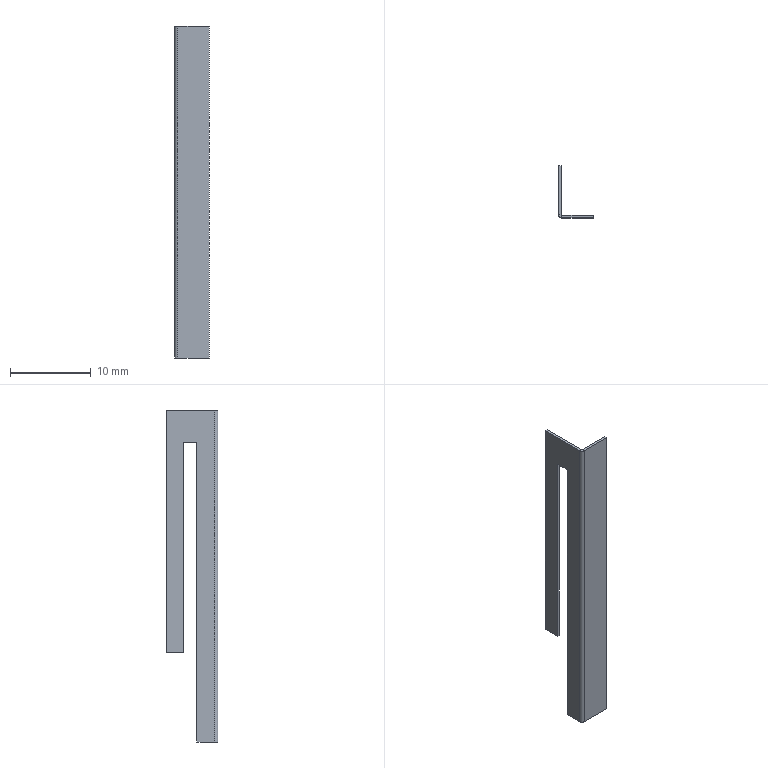Part | SolidWorks | features EdgeFlange 1, FlatPattern 1, SMBaseFlange 1, SheetMetal 1 | 1 solid | 18 faces | box 4.3 x 6.4 x 41 mm | volume 101.19 mm3 | plane 16 | cylinder 2 | commonest cylinder face diameters 0.2 x1 0.8 x1
STEP:
#1=CARTESIAN_POINT('',(3.9,0.,-41.));
#2=VERTEX_POINT('',#1);
#3=CARTESIAN_POINT('',(0.,0.,-41.));
#4=VERTEX_POINT('',#3);
#5=CARTESIAN_POINT('',(0.,0.,-41.));
#6=DIRECTION('',(-1.,0.,0.));
#7=VECTOR('',#6,1000.);
#8=LINE('',#5,#7);
#9=EDGE_CURVE('',#2,#4,#8,.T.);
#10=ORIENTED_EDGE('',*,*,#9,.F.);
#11=CARTESIAN_POINT('',(3.9,-0.3,-41.));
#12=VERTEX_POINT('',#11);
#13=CARTESIAN_POINT('',(3.9,-0.3,-41.));
#14=DIRECTION('',(0.,1.,0.));
#15=VECTOR('',#14,1000.);
#16=LINE('',#13,#15);
#17=EDGE_CURVE('',#12,#2,#16,.T.);
#18=ORIENTED_EDGE('',*,*,#17,.F.);
#19=CARTESIAN_POINT('',(0.,-0.3,-41.));
#20=VERTEX_POINT('',#19);
#21=CARTESIAN_POINT('',(0.,-0.3,-41.));
#22=DIRECTION('',(-1.,0.,0.));
#23=VECTOR('',#22,1000.);
#24=LINE('',#21,#23);
#25=EDGE_CURVE('',#12,#20,#24,.T.);
#26=ORIENTED_EDGE('',*,*,#25,.T.);
#27=CARTESIAN_POINT('',(0.,-0.3,-41.));
#28=DIRECTION('',(0.,1.,0.));
#29=VECTOR('',#28,1000.);
#30=LINE('',#27,#29);
#31=EDGE_CURVE('',#20,#4,#30,.T.);
#32=ORIENTED_EDGE('',*,*,#31,.T.);
#33=EDGE_LOOP('',(#10,#18,#26,#32));
#34=FACE_OUTER_BOUND('',#33,.T.);
#35=CARTESIAN_POINT('',(0.,-0.3,-41.));
#36=DIRECTION('',(0.,0.,-1.));
#37=DIRECTION('',(-1.,0.,0.));
#38=AXIS2_PLACEMENT_3D('',#35,#36,#37);
#39=PLANE('',#38);
#40=ADVANCED_FACE('',(#34),#39,.T.);
#41=CARTESIAN_POINT('',(3.9,0.,0.));
#42=VERTEX_POINT('',#41);
#43=CARTESIAN_POINT('',(3.9,0.,0.));
#44=DIRECTION('',(0.,0.,-1.));
#45=VECTOR('',#44,1000.);
#46=LINE('',#43,#45);
#47=EDGE_CURVE('',#42,#2,#46,.T.);
#48=ORIENTED_EDGE('',*,*,#47,.F.);
#49=CARTESIAN_POINT('',(3.9,-0.3,0.));
#50=VERTEX_POINT('',#49);
#51=CARTESIAN_POINT('',(3.9,-0.3,0.));
#52=DIRECTION('',(0.,1.,0.));
#53=VECTOR('',#52,1000.);
#54=LINE('',#51,#53);
#55=EDGE_CURVE('',#50,#42,#54,.T.);
#56=ORIENTED_EDGE('',*,*,#55,.F.);
#57=CARTESIAN_POINT('',(3.9,-0.3,0.));
#58=DIRECTION('',(0.,0.,-1.));
#59=VECTOR('',#58,1000.);
#60=LINE('',#57,#59);
#61=EDGE_CURVE('',#50,#12,#60,.T.);
#62=ORIENTED_EDGE('',*,*,#61,.T.);
#63=ORIENTED_EDGE('',*,*,#17,.T.);
#64=EDGE_LOOP('',(#48,#56,#62,#63));
#65=FACE_OUTER_BOUND('',#64,.T.);
#66=CARTESIAN_POINT('',(3.9,-0.3,0.));
#67=DIRECTION('',(1.,0.,0.));
#68=DIRECTION('',(0.,0.,-1.));
#69=AXIS2_PLACEMENT_3D('',#66,#67,#68);
#70=PLANE('',#69);
#71=ADVANCED_FACE('',(#65),#70,.T.);
#72=CARTESIAN_POINT('',(0.,0.,0.));
#73=VERTEX_POINT('',#72);
#74=CARTESIAN_POINT('',(0.,0.,0.));
#75=DIRECTION('',(1.,0.,0.));
#76=VECTOR('',#75,1000.);
#77=LINE('',#74,#76);
#78=EDGE_CURVE('',#73,#42,#77,.T.);
#79=ORIENTED_EDGE('',*,*,#78,.F.);
#80=CARTESIAN_POINT('',(0.,-0.3,0.));
#81=VERTEX_POINT('',#80);
#82=CARTESIAN_POINT('',(0.,-0.3,0.));
#83=DIRECTION('',(0.,1.,0.));
#84=VECTOR('',#83,1000.);
#85=LINE('',#82,#84);
#86=EDGE_CURVE('',#81,#73,#85,.T.);
#87=ORIENTED_EDGE('',*,*,#86,.F.);
#88=CARTESIAN_POINT('',(0.,-0.3,0.));
#89=DIRECTION('',(1.,0.,0.));
#90=VECTOR('',#89,1000.);
#91=LINE('',#88,#90);
#92=EDGE_CURVE('',#81,#50,#91,.T.);
#93=ORIENTED_EDGE('',*,*,#92,.T.);
#94=ORIENTED_EDGE('',*,*,#55,.T.);
#95=EDGE_LOOP('',(#79,#87,#93,#94));
#96=FACE_OUTER_BOUND('',#95,.T.);
#97=CARTESIAN_POINT('',(0.,-0.3,0.));
#98=DIRECTION('',(0.,0.,1.));
#99=DIRECTION('',(1.,0.,0.));
#100=AXIS2_PLACEMENT_3D('',#97,#98,#99);
#101=PLANE('',#100);
#102=ADVANCED_FACE('',(#96),#101,.T.);
#103=CARTESIAN_POINT('',(0.,-0.3,0.));
#104=DIRECTION('',(0.,0.,1.));
#105=VECTOR('',#104,1000.);
#106=LINE('',#103,#105);
#107=EDGE_CURVE('',#20,#81,#106,.T.);
#108=ORIENTED_EDGE('',*,*,#107,.F.);
#109=ORIENTED_EDGE('',*,*,#25,.F.);
#110=ORIENTED_EDGE('',*,*,#61,.F.);
#111=ORIENTED_EDGE('',*,*,#92,.F.);
#112=EDGE_LOOP('',(#108,#109,#110,#111));
#113=FACE_OUTER_BOUND('',#112,.T.);
#114=CARTESIAN_POINT('',(0.,-0.3,0.));
#115=DIRECTION('',(0.,-1.,0.));
#116=DIRECTION('',(0.,0.,-1.));
#117=AXIS2_PLACEMENT_3D('',#114,#115,#116);
#118=PLANE('',#117);
#119=ADVANCED_FACE('',(#113),#118,.T.);
#120=CARTESIAN_POINT('',(0.,0.,0.));
#121=DIRECTION('',(0.,0.,1.));
#122=VECTOR('',#121,1000.);
#123=LINE('',#120,#122);
#124=EDGE_CURVE('',#4,#73,#123,.T.);
#125=ORIENTED_EDGE('',*,*,#124,.T.);
#126=ORIENTED_EDGE('',*,*,#78,.T.);
#127=ORIENTED_EDGE('',*,*,#47,.T.);
#128=ORIENTED_EDGE('',*,*,#9,.T.);
#129=EDGE_LOOP('',(#125,#126,#127,#128));
#130=FACE_OUTER_BOUND('',#129,.T.);
#131=CARTESIAN_POINT('',(0.,0.,0.));
#132=DIRECTION('',(0.,-1.,0.));
#133=DIRECTION('',(0.,0.,-1.));
#134=AXIS2_PLACEMENT_3D('',#131,#132,#133);
#135=PLANE('',#134);
#136=ADVANCED_FACE('',(#130),#135,.F.);
#137=CARTESIAN_POINT('',(-0.1,0.1,-41.));
#138=VERTEX_POINT('',#137);
#139=CARTESIAN_POINT('',(-0.4,0.1,-41.));
#140=VERTEX_POINT('',#139);
#141=CARTESIAN_POINT('',(-0.4,0.1,-41.));
#142=DIRECTION('',(-1.,0.,0.));
#143=VECTOR('',#142,1000.);
#144=LINE('',#141,#143);
#145=EDGE_CURVE('',#138,#140,#144,.T.);
#146=ORIENTED_EDGE('',*,*,#145,.F.);
#147=CARTESIAN_POINT('',(0.,0.1,-41.));
#148=DIRECTION('',(0.,0.,-1.));
#149=DIRECTION('',(1.,0.,0.));
#150=AXIS2_PLACEMENT_3D('',#147,#148,#149);
#151=CIRCLE('',#150,0.1);
#152=EDGE_CURVE('',#4,#138,#151,.T.);
#153=ORIENTED_EDGE('',*,*,#152,.F.);
#154=ORIENTED_EDGE('',*,*,#31,.F.);
#155=CARTESIAN_POINT('',(0.,0.1,-41.));
#156=DIRECTION('',(0.,0.,-1.));
#157=DIRECTION('',(1.,0.,0.));
#158=AXIS2_PLACEMENT_3D('',#155,#156,#157);
#159=CIRCLE('',#158,0.4);
#160=EDGE_CURVE('',#20,#140,#159,.T.);
#161=ORIENTED_EDGE('',*,*,#160,.T.);
#162=EDGE_LOOP('',(#146,#153,#154,#161));
#163=FACE_OUTER_BOUND('',#162,.T.);
#164=CARTESIAN_POINT('',(0.,0.1,-41.));
#165=DIRECTION('',(0.,0.,-1.));
#166=DIRECTION('',(-1.,0.,0.));
#167=AXIS2_PLACEMENT_3D('',#164,#165,#166);
#168=PLANE('',#167);
#169=ADVANCED_FACE('',(#163),#168,.T.);
#170=CARTESIAN_POINT('',(-0.1,0.1,0.));
#171=VERTEX_POINT('',#170);
#172=CARTESIAN_POINT('',(0.,0.1,0.));
#173=DIRECTION('',(0.,0.,1.));
#174=DIRECTION('',(1.,0.,0.));
#175=AXIS2_PLACEMENT_3D('',#172,#173,#174);
#176=CIRCLE('',#175,0.1);
#177=EDGE_CURVE('',#171,#73,#176,.T.);
#178=ORIENTED_EDGE('',*,*,#177,.F.);
#179=CARTESIAN_POINT('',(-0.4,0.1,0.));
#180=VERTEX_POINT('',#179);
#181=CARTESIAN_POINT('',(-0.1,0.1,0.));
#182=DIRECTION('',(-1.,0.,0.));
#183=VECTOR('',#182,1000.);
#184=LINE('',#181,#183);
#185=EDGE_CURVE('',#171,#180,#184,.T.);
#186=ORIENTED_EDGE('',*,*,#185,.T.);
#187=CARTESIAN_POINT('',(0.,0.1,0.));
#188=DIRECTION('',(0.,0.,1.));
#189=DIRECTION('',(1.,0.,0.));
#190=AXIS2_PLACEMENT_3D('',#187,#188,#189);
#191=CIRCLE('',#190,0.4);
#192=EDGE_CURVE('',#180,#81,#191,.T.);
#193=ORIENTED_EDGE('',*,*,#192,.T.);
#194=ORIENTED_EDGE('',*,*,#86,.T.);
#195=EDGE_LOOP('',(#178,#186,#193,#194));
#196=FACE_OUTER_BOUND('',#195,.T.);
#197=CARTESIAN_POINT('',(0.,0.1,0.));
#198=DIRECTION('',(0.,0.,-1.));
#199=DIRECTION('',(-1.,0.,0.));
#200=AXIS2_PLACEMENT_3D('',#197,#198,#199);
#201=PLANE('',#200);
#202=ADVANCED_FACE('',(#196),#201,.F.);
#203=ORIENTED_EDGE('',*,*,#107,.T.);
#204=ORIENTED_EDGE('',*,*,#192,.F.);
#205=CARTESIAN_POINT('',(-0.4,0.1,-41.));
#206=DIRECTION('',(0.,0.,-1.));
#207=VECTOR('',#206,1000.);
#208=LINE('',#205,#207);
#209=EDGE_CURVE('',#180,#140,#208,.T.);
#210=ORIENTED_EDGE('',*,*,#209,.T.);
#211=ORIENTED_EDGE('',*,*,#160,.F.);
#212=EDGE_LOOP('',(#203,#204,#210,#211));
#213=FACE_OUTER_BOUND('',#212,.T.);
#214=CARTESIAN_POINT('',(0.,0.1,0.));
#215=DIRECTION('',(0.,0.,1.));
#216=DIRECTION('',(-1.,0.,0.));
#217=AXIS2_PLACEMENT_3D('',#214,#215,#216);
#218=CYLINDRICAL_SURFACE('',#217,0.4);
#219=ADVANCED_FACE('',(#213),#218,.T.);
#220=ORIENTED_EDGE('',*,*,#124,.F.);
#221=ORIENTED_EDGE('',*,*,#152,.T.);
#222=CARTESIAN_POINT('',(-0.1,0.1,-41.));
#223=DIRECTION('',(0.,0.,1.));
#224=VECTOR('',#223,1000.);
#225=LINE('',#222,#224);
#226=EDGE_CURVE('',#138,#171,#225,.T.);
#227=ORIENTED_EDGE('',*,*,#226,.T.);
#228=ORIENTED_EDGE('',*,*,#177,.T.);
#229=EDGE_LOOP('',(#220,#221,#227,#228));
#230=FACE_OUTER_BOUND('',#229,.T.);
#231=CARTESIAN_POINT('',(0.,0.1,0.));
#232=DIRECTION('',(0.,0.,1.));
#233=DIRECTION('',(-1.,0.,0.));
#234=AXIS2_PLACEMENT_3D('',#231,#232,#233);
#235=CYLINDRICAL_SURFACE('',#234,0.1);
#236=ADVANCED_FACE('',(#230),#235,.F.);
#237=ORIENTED_EDGE('',*,*,#145,.T.);
#238=CARTESIAN_POINT('',(-0.4,2.3,-41.));
#239=VERTEX_POINT('',#238);
#240=CARTESIAN_POINT('',(-0.4,0.,-41.));
#241=DIRECTION('',(0.,-1.,0.));
#242=VECTOR('',#241,1000.);
#243=LINE('',#240,#242);
#244=EDGE_CURVE('',#239,#140,#243,.T.);
#245=ORIENTED_EDGE('',*,*,#244,.F.);
#246=CARTESIAN_POINT('',(-0.1,2.3,-41.));
#247=VERTEX_POINT('',#246);
#248=CARTESIAN_POINT('',(-0.4,2.3,-41.));
#249=DIRECTION('',(1.,0.,0.));
#250=VECTOR('',#249,1000.);
#251=LINE('',#248,#250);
#252=EDGE_CURVE('',#239,#247,#251,.T.);
#253=ORIENTED_EDGE('',*,*,#252,.T.);
#254=CARTESIAN_POINT('',(-0.1,0.,-41.));
#255=DIRECTION('',(0.,-1.,0.));
#256=VECTOR('',#255,1000.);
#257=LINE('',#254,#256);
#258=EDGE_CURVE('',#247,#138,#257,.T.);
#259=ORIENTED_EDGE('',*,*,#258,.T.);
#260=EDGE_LOOP('',(#237,#245,#253,#259));
#261=FACE_OUTER_BOUND('',#260,.T.);
#262=CARTESIAN_POINT('',(-0.4,0.,-41.));
#263=DIRECTION('',(0.,0.,1.));
#264=DIRECTION('',(1.,0.,0.));
#265=AXIS2_PLACEMENT_3D('',#262,#263,#264);
#266=PLANE('',#265);
#267=ADVANCED_FACE('',(#261),#266,.F.);
#268=ORIENTED_EDGE('',*,*,#185,.F.);
#269=CARTESIAN_POINT('',(-0.1,6.1,0.));
#270=VERTEX_POINT('',#269);
#271=CARTESIAN_POINT('',(-0.1,6.1,0.));
#272=DIRECTION('',(0.,1.,0.));
#273=VECTOR('',#272,1000.);
#274=LINE('',#271,#273);
#275=EDGE_CURVE('',#171,#270,#274,.T.);
#276=ORIENTED_EDGE('',*,*,#275,.T.);
#277=CARTESIAN_POINT('',(-0.4,6.1,0.));
#278=VERTEX_POINT('',#277);
#279=CARTESIAN_POINT('',(-0.4,6.1,0.));
#280=DIRECTION('',(1.,0.,0.));
#281=VECTOR('',#280,1000.);
#282=LINE('',#279,#281);
#283=EDGE_CURVE('',#278,#270,#282,.T.);
#284=ORIENTED_EDGE('',*,*,#283,.F.);
#285=CARTESIAN_POINT('',(-0.4,0.,0.));
#286=DIRECTION('',(0.,1.,0.));
#287=VECTOR('',#286,1000.);
#288=LINE('',#285,#287);
#289=EDGE_CURVE('',#180,#278,#288,.T.);
#290=ORIENTED_EDGE('',*,*,#289,.F.);
#291=EDGE_LOOP('',(#268,#276,#284,#290));
#292=FACE_OUTER_BOUND('',#291,.T.);
#293=CARTESIAN_POINT('',(-0.4,6.1,0.));
#294=DIRECTION('',(0.,0.,-1.));
#295=DIRECTION('',(0.,1.,0.));
#296=AXIS2_PLACEMENT_3D('',#293,#294,#295);
#297=PLANE('',#296);
#298=ADVANCED_FACE('',(#292),#297,.F.);
#299=ORIENTED_EDGE('',*,*,#209,.F.);
#300=ORIENTED_EDGE('',*,*,#289,.T.);
#301=CARTESIAN_POINT('',(-0.4,6.1,-30.));
#302=VERTEX_POINT('',#301);
#303=CARTESIAN_POINT('',(-0.4,6.1,0.));
#304=DIRECTION('',(0.,0.,-1.));
#305=VECTOR('',#304,1000.);
#306=LINE('',#303,#305);
#307=EDGE_CURVE('',#278,#302,#306,.T.);
#308=ORIENTED_EDGE('',*,*,#307,.T.);
#309=CARTESIAN_POINT('',(-0.4,3.95,-30.));
#310=VERTEX_POINT('',#309);
#311=CARTESIAN_POINT('',(-0.4,0.,-30.));
#312=DIRECTION('',(0.,-1.,0.));
#313=VECTOR('',#312,1000.);
#314=LINE('',#311,#313);
#315=EDGE_CURVE('',#302,#310,#314,.T.);
#316=ORIENTED_EDGE('',*,*,#315,.T.);
#317=CARTESIAN_POINT('',(-0.4,3.95,-4.));
#318=VERTEX_POINT('',#317);
#319=CARTESIAN_POINT('',(-0.4,3.95,0.));
#320=DIRECTION('',(0.,0.,1.));
#321=VECTOR('',#320,1000.);
#322=LINE('',#319,#321);
#323=EDGE_CURVE('',#310,#318,#322,.T.);
#324=ORIENTED_EDGE('',*,*,#323,.T.);
#325=CARTESIAN_POINT('',(-0.4,2.3,-4.));
#326=VERTEX_POINT('',#325);
#327=CARTESIAN_POINT('',(-0.4,0.,-4.));
#328=DIRECTION('',(0.,-1.,0.));
#329=VECTOR('',#328,1000.);
#330=LINE('',#327,#329);
#331=EDGE_CURVE('',#318,#326,#330,.T.);
#332=ORIENTED_EDGE('',*,*,#331,.T.);
#333=CARTESIAN_POINT('',(-0.4,2.3,0.));
#334=DIRECTION('',(0.,0.,-1.));
#335=VECTOR('',#334,1000.);
#336=LINE('',#333,#335);
#337=EDGE_CURVE('',#326,#239,#336,.T.);
#338=ORIENTED_EDGE('',*,*,#337,.T.);
#339=ORIENTED_EDGE('',*,*,#244,.T.);
#340=EDGE_LOOP('',(#299,#300,#308,#316,#324,#332,#338,#339));
#341=FACE_OUTER_BOUND('',#340,.T.);
#342=CARTESIAN_POINT('',(-0.4,0.,0.));
#343=DIRECTION('',(1.,0.,0.));
#344=DIRECTION('',(0.,1.,0.));
#345=AXIS2_PLACEMENT_3D('',#342,#343,#344);
#346=PLANE('',#345);
#347=ADVANCED_FACE('',(#341),#346,.F.);
#348=ORIENTED_EDGE('',*,*,#275,.F.);
#349=ORIENTED_EDGE('',*,*,#226,.F.);
#350=ORIENTED_EDGE('',*,*,#258,.F.);
#351=CARTESIAN_POINT('',(-0.1,2.3,-4.));
#352=VERTEX_POINT('',#351);
#353=CARTESIAN_POINT('',(-0.1,2.3,-41.));
#354=DIRECTION('',(0.,0.,-1.));
#355=VECTOR('',#354,1000.);
#356=LINE('',#353,#355);
#357=EDGE_CURVE('',#352,#247,#356,.T.);
#358=ORIENTED_EDGE('',*,*,#357,.F.);
#359=CARTESIAN_POINT('',(-0.1,3.95,-4.));
#360=VERTEX_POINT('',#359);
#361=CARTESIAN_POINT('',(-0.1,2.3,-4.));
#362=DIRECTION('',(0.,-1.,0.));
#363=VECTOR('',#362,1000.);
#364=LINE('',#361,#363);
#365=EDGE_CURVE('',#360,#352,#364,.T.);
#366=ORIENTED_EDGE('',*,*,#365,.F.);
#367=CARTESIAN_POINT('',(-0.1,3.95,-30.));
#368=VERTEX_POINT('',#367);
#369=CARTESIAN_POINT('',(-0.1,3.95,-4.));
#370=DIRECTION('',(0.,0.,1.));
#371=VECTOR('',#370,1000.);
#372=LINE('',#369,#371);
#373=EDGE_CURVE('',#368,#360,#372,.T.);
#374=ORIENTED_EDGE('',*,*,#373,.F.);
#375=CARTESIAN_POINT('',(-0.1,6.1,-30.));
#376=VERTEX_POINT('',#375);
#377=CARTESIAN_POINT('',(-0.1,3.95,-30.));
#378=DIRECTION('',(0.,-1.,0.));
#379=VECTOR('',#378,1000.);
#380=LINE('',#377,#379);
#381=EDGE_CURVE('',#376,#368,#380,.T.);
#382=ORIENTED_EDGE('',*,*,#381,.F.);
#383=CARTESIAN_POINT('',(-0.1,6.1,-30.));
#384=DIRECTION('',(0.,0.,-1.));
#385=VECTOR('',#384,1000.);
#386=LINE('',#383,#385);
#387=EDGE_CURVE('',#270,#376,#386,.T.);
#388=ORIENTED_EDGE('',*,*,#387,.F.);
#389=EDGE_LOOP('',(#348,#349,#350,#358,#366,#374,#382,#388));
#390=FACE_OUTER_BOUND('',#389,.T.);
#391=CARTESIAN_POINT('',(-0.1,0.,0.));
#392=DIRECTION('',(1.,0.,0.));
#393=DIRECTION('',(0.,1.,0.));
#394=AXIS2_PLACEMENT_3D('',#391,#392,#393);
#395=PLANE('',#394);
#396=ADVANCED_FACE('',(#390),#395,.T.);
#397=ORIENTED_EDGE('',*,*,#387,.T.);
#398=CARTESIAN_POINT('',(-0.4,6.1,-30.));
#399=DIRECTION('',(1.,0.,0.));
#400=VECTOR('',#399,1000.);
#401=LINE('',#398,#400);
#402=EDGE_CURVE('',#302,#376,#401,.T.);
#403=ORIENTED_EDGE('',*,*,#402,.F.);
#404=ORIENTED_EDGE('',*,*,#307,.F.);
#405=ORIENTED_EDGE('',*,*,#283,.T.);
#406=EDGE_LOOP('',(#397,#403,#404,#405));
#407=FACE_OUTER_BOUND('',#406,.T.);
#408=CARTESIAN_POINT('',(-0.4,6.1,-30.));
#409=DIRECTION('',(0.,-1.,0.));
#410=DIRECTION('',(1.,0.,0.));
#411=AXIS2_PLACEMENT_3D('',#408,#409,#410);
#412=PLANE('',#411);
#413=ADVANCED_FACE('',(#407),#412,.F.);
#414=ORIENTED_EDGE('',*,*,#381,.T.);
#415=CARTESIAN_POINT('',(-0.4,3.95,-30.));
#416=DIRECTION('',(1.,0.,0.));
#417=VECTOR('',#416,1000.);
#418=LINE('',#415,#417);
#419=EDGE_CURVE('',#310,#368,#418,.T.);
#420=ORIENTED_EDGE('',*,*,#419,.F.);
#421=ORIENTED_EDGE('',*,*,#315,.F.);
#422=ORIENTED_EDGE('',*,*,#402,.T.);
#423=EDGE_LOOP('',(#414,#420,#421,#422));
#424=FACE_OUTER_BOUND('',#423,.T.);
#425=CARTESIAN_POINT('',(-0.4,3.95,-30.));
#426=DIRECTION('',(0.,0.,1.));
#427=DIRECTION('',(1.,0.,0.));
#428=AXIS2_PLACEMENT_3D('',#425,#426,#427);
#429=PLANE('',#428);
#430=ADVANCED_FACE('',(#424),#429,.F.);
#431=ORIENTED_EDGE('',*,*,#373,.T.);
#432=CARTESIAN_POINT('',(-0.4,3.95,-4.));
#433=DIRECTION('',(1.,0.,0.));
#434=VECTOR('',#433,1000.);
#435=LINE('',#432,#434);
#436=EDGE_CURVE('',#318,#360,#435,.T.);
#437=ORIENTED_EDGE('',*,*,#436,.F.);
#438=ORIENTED_EDGE('',*,*,#323,.F.);
#439=ORIENTED_EDGE('',*,*,#419,.T.);
#440=EDGE_LOOP('',(#431,#437,#438,#439));
#441=FACE_OUTER_BOUND('',#440,.T.);
#442=CARTESIAN_POINT('',(-0.4,3.95,-4.));
#443=DIRECTION('',(0.,1.,0.));
#444=DIRECTION('',(-1.,0.,0.));
#445=AXIS2_PLACEMENT_3D('',#442,#443,#444);
#446=PLANE('',#445);
#447=ADVANCED_FACE('',(#441),#446,.F.);
#448=ORIENTED_EDGE('',*,*,#365,.T.);
#449=CARTESIAN_POINT('',(-0.4,2.3,-4.));
#450=DIRECTION('',(1.,0.,0.));
#451=VECTOR('',#450,1000.);
#452=LINE('',#449,#451);
#453=EDGE_CURVE('',#326,#352,#452,.T.);
#454=ORIENTED_EDGE('',*,*,#453,.F.);
#455=ORIENTED_EDGE('',*,*,#331,.F.);
#456=ORIENTED_EDGE('',*,*,#436,.T.);
#457=EDGE_LOOP('',(#448,#454,#455,#456));
#458=FACE_OUTER_BOUND('',#457,.T.);
#459=CARTESIAN_POINT('',(-0.4,2.3,-4.));
#460=DIRECTION('',(0.,0.,1.));
#461=DIRECTION('',(0.,-1.,0.));
#462=AXIS2_PLACEMENT_3D('',#459,#460,#461);
#463=PLANE('',#462);
#464=ADVANCED_FACE('',(#458),#463,.F.);
#465=ORIENTED_EDGE('',*,*,#357,.T.);
#466=ORIENTED_EDGE('',*,*,#252,.F.);
#467=ORIENTED_EDGE('',*,*,#337,.F.);
#468=ORIENTED_EDGE('',*,*,#453,.T.);
#469=EDGE_LOOP('',(#465,#466,#467,#468));
#470=FACE_OUTER_BOUND('',#469,.T.);
#471=CARTESIAN_POINT('',(-0.4,2.3,-41.));
#472=DIRECTION('',(0.,-1.,0.));
#473=DIRECTION('',(1.,0.,0.));
#474=AXIS2_PLACEMENT_3D('',#471,#472,#473);
#475=PLANE('',#474);
#476=ADVANCED_FACE('',(#470),#475,.F.);
#477=CLOSED_SHELL('',(#40,#71,#102,#119,#136,#169,#202,#219,#236,#267,#298,#347,#396,#413,#430,#447,#464,#476));
#478=MANIFOLD_SOLID_BREP('',#477);
#479=CARTESIAN_POINT('',(0.,0.,0.));
#480=DIRECTION('',(0.,0.,1.));
#481=DIRECTION('',(1.,0.,0.));
#482=AXIS2_PLACEMENT_3D('',#479,#480,#481);
#483=(LENGTH_UNIT()NAMED_UNIT(*)SI_UNIT(.MILLI.,.METRE.));
#484=UNCERTAINTY_MEASURE_WITH_UNIT(LENGTH_MEASURE(0.00001),#483,'','');
#485=(NAMED_UNIT(*)PLANE_ANGLE_UNIT()SI_UNIT($,.RADIAN.));
#486=(NAMED_UNIT(*)SI_UNIT($,.STERADIAN.)SOLID_ANGLE_UNIT());
#487=(GEOMETRIC_REPRESENTATION_CONTEXT(3)GLOBAL_UNCERTAINTY_ASSIGNED_CONTEXT((#484))GLOBAL_UNIT_ASSIGNED_CONTEXT((#483,#485,#486))REPRESENTATION_CONTEXT('',''));
#488=ADVANCED_BREP_SHAPE_REPRESENTATION('',(#478,#482),#487);